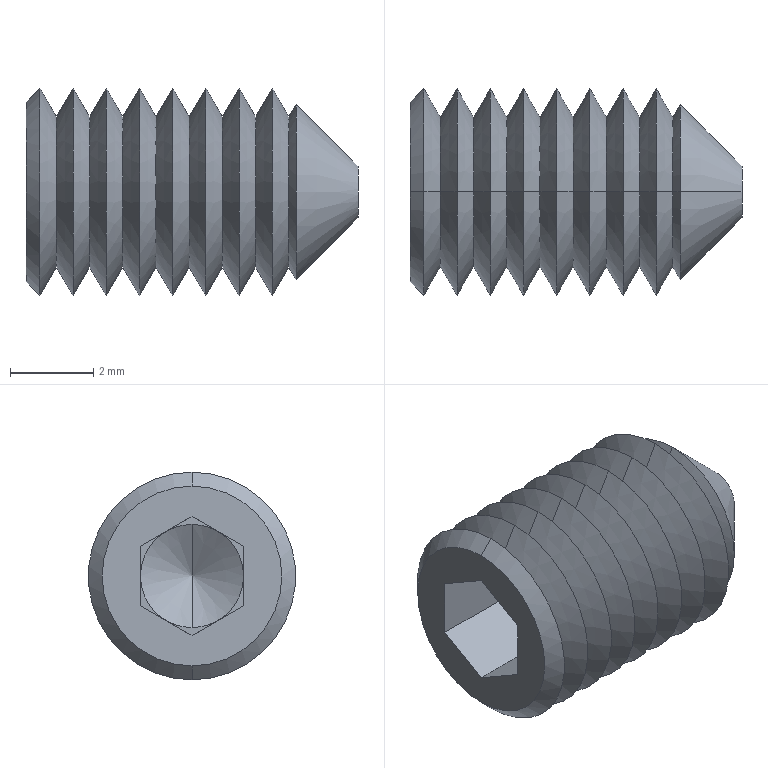Part | STEP file | GB/T 78 M5×8 | 1 solid | 52 faces | box 8 x 5 x 5 mm | volume 93.812 mm3 | cone 38 | plane 14
STEP:
#1=CARTESIAN_POINT('',(8.,0.,0.625));
#2=VERTEX_POINT('',#1);
#3=CARTESIAN_POINT('',(8.,0.,-0.625));
#4=VERTEX_POINT('',#3);
#5=CARTESIAN_POINT('',(8.,0.,0.));
#6=DIRECTION('',(-1.,0.,0.));
#7=DIRECTION('',(0.,0.,1.));
#8=AXIS2_PLACEMENT_3D('',#5,#6,#7);
#9=CIRCLE('',#8,0.625);
#10=EDGE_CURVE('',#2,#4,#9,.T.);
#11=ORIENTED_EDGE('',*,*,#10,.T.);
#12=CARTESIAN_POINT('',(6.51,0.,-2.115));
#13=VERTEX_POINT('',#12);
#14=CARTESIAN_POINT('',(8.,0.,-0.625));
#15=DIRECTION('',(-0.7071,0.,-0.7071));
#16=VECTOR('',#15,1000.);
#17=LINE('',#14,#16);
#18=EDGE_CURVE('',#4,#13,#17,.T.);
#19=ORIENTED_EDGE('',*,*,#18,.T.);
#20=CARTESIAN_POINT('',(6.51,0.,2.115));
#21=VERTEX_POINT('',#20);
#22=CARTESIAN_POINT('',(6.51,0.,0.));
#23=DIRECTION('',(-1.,0.,0.));
#24=DIRECTION('',(0.,0.,-1.));
#25=AXIS2_PLACEMENT_3D('',#22,#23,#24);
#26=CIRCLE('',#25,2.115);
#27=EDGE_CURVE('',#21,#13,#26,.T.);
#28=ORIENTED_EDGE('',*,*,#27,.F.);
#29=CARTESIAN_POINT('',(8.,0.,0.625));
#30=DIRECTION('',(-0.7071,0.,0.7071));
#31=VECTOR('',#30,1000.);
#32=LINE('',#29,#31);
#33=EDGE_CURVE('',#2,#21,#32,.T.);
#34=ORIENTED_EDGE('',*,*,#33,.F.);
#35=EDGE_LOOP('',(#11,#19,#28,#34));
#36=FACE_OUTER_BOUND('',#35,.T.);
#37=CARTESIAN_POINT('',(8.,0.,0.));
#38=DIRECTION('',(-1.,0.,0.));
#39=DIRECTION('',(0.,0.,1.));
#40=AXIS2_PLACEMENT_3D('',#37,#38,#39);
#41=CONICAL_SURFACE('',#40,0.625,0.7854);
#42=ADVANCED_FACE('',(#36),#41,.T.);
#43=CARTESIAN_POINT('',(6.331,0.,1.807));
#44=VERTEX_POINT('',#43);
#45=CARTESIAN_POINT('',(6.331,0.,-1.807));
#46=VERTEX_POINT('',#45);
#47=CARTESIAN_POINT('',(6.331,0.,0.));
#48=DIRECTION('',(-1.,0.,0.));
#49=DIRECTION('',(0.,0.,1.));
#50=AXIS2_PLACEMENT_3D('',#47,#48,#49);
#51=CIRCLE('',#50,1.807);
#52=EDGE_CURVE('',#44,#46,#51,.T.);
#53=ORIENTED_EDGE('',*,*,#52,.T.);
#54=CARTESIAN_POINT('',(5.935,0.,-2.5));
#55=VERTEX_POINT('',#54);
#56=CARTESIAN_POINT('',(5.935,0.,-2.5));
#57=DIRECTION('',(-0.4959,0.,-0.8684));
#58=VECTOR('',#57,1000.);
#59=LINE('',#56,#58);
#60=EDGE_CURVE('',#46,#55,#59,.T.);
#61=ORIENTED_EDGE('',*,*,#60,.T.);
#62=CARTESIAN_POINT('',(5.935,0.,2.5));
#63=VERTEX_POINT('',#62);
#64=CARTESIAN_POINT('',(5.935,0.,0.));
#65=DIRECTION('',(-1.,0.,0.));
#66=DIRECTION('',(0.,0.,1.));
#67=AXIS2_PLACEMENT_3D('',#64,#65,#66);
#68=CIRCLE('',#67,2.5);
#69=EDGE_CURVE('',#63,#55,#68,.T.);
#70=ORIENTED_EDGE('',*,*,#69,.F.);
#71=CARTESIAN_POINT('',(5.935,0.,2.5));
#72=DIRECTION('',(-0.4959,0.,0.8684));
#73=VECTOR('',#72,1000.);
#74=LINE('',#71,#73);
#75=EDGE_CURVE('',#44,#63,#74,.T.);
#76=ORIENTED_EDGE('',*,*,#75,.F.);
#77=EDGE_LOOP('',(#53,#61,#70,#76));
#78=FACE_OUTER_BOUND('',#77,.T.);
#79=CARTESIAN_POINT('',(5.935,0.,0.));
#80=DIRECTION('',(-1.,0.,0.));
#81=DIRECTION('',(0.,0.,1.));
#82=AXIS2_PLACEMENT_3D('',#79,#80,#81);
#83=CONICAL_SURFACE('',#82,2.5,1.052);
#84=ADVANCED_FACE('',(#78),#83,.T.);
#85=ORIENTED_EDGE('',*,*,#52,.F.);
#86=CARTESIAN_POINT('',(6.331,0.,1.807));
#87=DIRECTION('',(0.5041,0.,0.8637));
#88=VECTOR('',#87,1000.);
#89=LINE('',#86,#88);
#90=EDGE_CURVE('',#44,#21,#89,.T.);
#91=ORIENTED_EDGE('',*,*,#90,.T.);
#92=ORIENTED_EDGE('',*,*,#27,.T.);
#93=CARTESIAN_POINT('',(6.331,0.,-1.807));
#94=DIRECTION('',(0.5041,0.,-0.8637));
#95=VECTOR('',#94,1000.);
#96=LINE('',#93,#95);
#97=EDGE_CURVE('',#46,#13,#96,.T.);
#98=ORIENTED_EDGE('',*,*,#97,.F.);
#99=EDGE_LOOP('',(#85,#91,#92,#98));
#100=FACE_OUTER_BOUND('',#99,.T.);
#101=CARTESIAN_POINT('',(6.331,0.,0.));
#102=DIRECTION('',(1.,0.,0.));
#103=DIRECTION('',(0.,0.,-1.));
#104=AXIS2_PLACEMENT_3D('',#101,#102,#103);
#105=CONICAL_SURFACE('',#104,1.807,1.043);
#106=ADVANCED_FACE('',(#100),#105,.T.);
#107=CARTESIAN_POINT('',(5.531,0.,1.807));
#108=VERTEX_POINT('',#107);
#109=CARTESIAN_POINT('',(5.531,0.,-1.807));
#110=VERTEX_POINT('',#109);
#111=CARTESIAN_POINT('',(5.531,0.,0.));
#112=DIRECTION('',(-1.,0.,0.));
#113=DIRECTION('',(0.,0.,1.));
#114=AXIS2_PLACEMENT_3D('',#111,#112,#113);
#115=CIRCLE('',#114,1.807);
#116=EDGE_CURVE('',#108,#110,#115,.T.);
#117=ORIENTED_EDGE('',*,*,#116,.F.);
#118=CARTESIAN_POINT('',(5.531,0.,1.807));
#119=DIRECTION('',(0.5041,0.,0.8637));
#120=VECTOR('',#119,1000.);
#121=LINE('',#118,#120);
#122=EDGE_CURVE('',#108,#63,#121,.T.);
#123=ORIENTED_EDGE('',*,*,#122,.T.);
#124=ORIENTED_EDGE('',*,*,#69,.T.);
#125=CARTESIAN_POINT('',(5.531,0.,-1.807));
#126=DIRECTION('',(0.5041,0.,-0.8637));
#127=VECTOR('',#126,1000.);
#128=LINE('',#125,#127);
#129=EDGE_CURVE('',#110,#55,#128,.T.);
#130=ORIENTED_EDGE('',*,*,#129,.F.);
#131=EDGE_LOOP('',(#117,#123,#124,#130));
#132=FACE_OUTER_BOUND('',#131,.T.);
#133=CARTESIAN_POINT('',(5.531,0.,0.));
#134=DIRECTION('',(1.,0.,0.));
#135=DIRECTION('',(0.,0.,-1.));
#136=AXIS2_PLACEMENT_3D('',#133,#134,#135);
#137=CONICAL_SURFACE('',#136,1.807,1.043);
#138=ADVANCED_FACE('',(#132),#137,.T.);
#139=ORIENTED_EDGE('',*,*,#116,.T.);
#140=CARTESIAN_POINT('',(5.135,0.,-2.5));
#141=VERTEX_POINT('',#140);
#142=CARTESIAN_POINT('',(5.135,0.,-2.5));
#143=DIRECTION('',(-0.4959,0.,-0.8684));
#144=VECTOR('',#143,1000.);
#145=LINE('',#142,#144);
#146=EDGE_CURVE('',#110,#141,#145,.T.);
#147=ORIENTED_EDGE('',*,*,#146,.T.);
#148=CARTESIAN_POINT('',(5.135,0.,2.5));
#149=VERTEX_POINT('',#148);
#150=CARTESIAN_POINT('',(5.135,0.,0.));
#151=DIRECTION('',(-1.,0.,0.));
#152=DIRECTION('',(0.,0.,1.));
#153=AXIS2_PLACEMENT_3D('',#150,#151,#152);
#154=CIRCLE('',#153,2.5);
#155=EDGE_CURVE('',#149,#141,#154,.T.);
#156=ORIENTED_EDGE('',*,*,#155,.F.);
#157=CARTESIAN_POINT('',(5.135,0.,2.5));
#158=DIRECTION('',(-0.4959,0.,0.8684));
#159=VECTOR('',#158,1000.);
#160=LINE('',#157,#159);
#161=EDGE_CURVE('',#108,#149,#160,.T.);
#162=ORIENTED_EDGE('',*,*,#161,.F.);
#163=EDGE_LOOP('',(#139,#147,#156,#162));
#164=FACE_OUTER_BOUND('',#163,.T.);
#165=CARTESIAN_POINT('',(5.135,0.,0.));
#166=DIRECTION('',(-1.,0.,0.));
#167=DIRECTION('',(0.,0.,1.));
#168=AXIS2_PLACEMENT_3D('',#165,#166,#167);
#169=CONICAL_SURFACE('',#168,2.5,1.052);
#170=ADVANCED_FACE('',(#164),#169,.T.);
#171=CARTESIAN_POINT('',(4.731,0.,1.807));
#172=VERTEX_POINT('',#171);
#173=CARTESIAN_POINT('',(4.731,0.,-1.807));
#174=VERTEX_POINT('',#173);
#175=CARTESIAN_POINT('',(4.731,0.,0.));
#176=DIRECTION('',(-1.,0.,0.));
#177=DIRECTION('',(0.,0.,1.));
#178=AXIS2_PLACEMENT_3D('',#175,#176,#177);
#179=CIRCLE('',#178,1.807);
#180=EDGE_CURVE('',#172,#174,#179,.T.);
#181=ORIENTED_EDGE('',*,*,#180,.F.);
#182=CARTESIAN_POINT('',(4.731,0.,1.807));
#183=DIRECTION('',(0.5041,0.,0.8637));
#184=VECTOR('',#183,1000.);
#185=LINE('',#182,#184);
#186=EDGE_CURVE('',#172,#149,#185,.T.);
#187=ORIENTED_EDGE('',*,*,#186,.T.);
#188=ORIENTED_EDGE('',*,*,#155,.T.);
#189=CARTESIAN_POINT('',(4.731,0.,-1.807));
#190=DIRECTION('',(0.5041,0.,-0.8637));
#191=VECTOR('',#190,1000.);
#192=LINE('',#189,#191);
#193=EDGE_CURVE('',#174,#141,#192,.T.);
#194=ORIENTED_EDGE('',*,*,#193,.F.);
#195=EDGE_LOOP('',(#181,#187,#188,#194));
#196=FACE_OUTER_BOUND('',#195,.T.);
#197=CARTESIAN_POINT('',(4.731,0.,0.));
#198=DIRECTION('',(1.,0.,0.));
#199=DIRECTION('',(0.,0.,-1.));
#200=AXIS2_PLACEMENT_3D('',#197,#198,#199);
#201=CONICAL_SURFACE('',#200,1.807,1.043);
#202=ADVANCED_FACE('',(#196),#201,.T.);
#203=ORIENTED_EDGE('',*,*,#180,.T.);
#204=CARTESIAN_POINT('',(4.335,0.,-2.5));
#205=VERTEX_POINT('',#204);
#206=CARTESIAN_POINT('',(4.335,0.,-2.5));
#207=DIRECTION('',(-0.4959,0.,-0.8684));
#208=VECTOR('',#207,1000.);
#209=LINE('',#206,#208);
#210=EDGE_CURVE('',#174,#205,#209,.T.);
#211=ORIENTED_EDGE('',*,*,#210,.T.);
#212=CARTESIAN_POINT('',(4.335,0.,2.5));
#213=VERTEX_POINT('',#212);
#214=CARTESIAN_POINT('',(4.335,0.,0.));
#215=DIRECTION('',(-1.,0.,0.));
#216=DIRECTION('',(0.,0.,1.));
#217=AXIS2_PLACEMENT_3D('',#214,#215,#216);
#218=CIRCLE('',#217,2.5);
#219=EDGE_CURVE('',#213,#205,#218,.T.);
#220=ORIENTED_EDGE('',*,*,#219,.F.);
#221=CARTESIAN_POINT('',(4.335,0.,2.5));
#222=DIRECTION('',(-0.4959,0.,0.8684));
#223=VECTOR('',#222,1000.);
#224=LINE('',#221,#223);
#225=EDGE_CURVE('',#172,#213,#224,.T.);
#226=ORIENTED_EDGE('',*,*,#225,.F.);
#227=EDGE_LOOP('',(#203,#211,#220,#226));
#228=FACE_OUTER_BOUND('',#227,.T.);
#229=CARTESIAN_POINT('',(4.335,0.,0.));
#230=DIRECTION('',(-1.,0.,0.));
#231=DIRECTION('',(0.,0.,1.));
#232=AXIS2_PLACEMENT_3D('',#229,#230,#231);
#233=CONICAL_SURFACE('',#232,2.5,1.052);
#234=ADVANCED_FACE('',(#228),#233,.T.);
#235=CARTESIAN_POINT('',(3.931,0.,1.807));
#236=VERTEX_POINT('',#235);
#237=CARTESIAN_POINT('',(3.931,0.,-1.807));
#238=VERTEX_POINT('',#237);
#239=CARTESIAN_POINT('',(3.931,0.,0.));
#240=DIRECTION('',(-1.,0.,0.));
#241=DIRECTION('',(0.,0.,1.));
#242=AXIS2_PLACEMENT_3D('',#239,#240,#241);
#243=CIRCLE('',#242,1.807);
#244=EDGE_CURVE('',#236,#238,#243,.T.);
#245=ORIENTED_EDGE('',*,*,#244,.F.);
#246=CARTESIAN_POINT('',(3.931,0.,1.807));
#247=DIRECTION('',(0.5041,0.,0.8637));
#248=VECTOR('',#247,1000.);
#249=LINE('',#246,#248);
#250=EDGE_CURVE('',#236,#213,#249,.T.);
#251=ORIENTED_EDGE('',*,*,#250,.T.);
#252=ORIENTED_EDGE('',*,*,#219,.T.);
#253=CARTESIAN_POINT('',(3.931,0.,-1.807));
#254=DIRECTION('',(0.5041,0.,-0.8637));
#255=VECTOR('',#254,1000.);
#256=LINE('',#253,#255);
#257=EDGE_CURVE('',#238,#205,#256,.T.);
#258=ORIENTED_EDGE('',*,*,#257,.F.);
#259=EDGE_LOOP('',(#245,#251,#252,#258));
#260=FACE_OUTER_BOUND('',#259,.T.);
#261=CARTESIAN_POINT('',(3.931,0.,0.));
#262=DIRECTION('',(1.,0.,0.));
#263=DIRECTION('',(0.,0.,-1.));
#264=AXIS2_PLACEMENT_3D('',#261,#262,#263);
#265=CONICAL_SURFACE('',#264,1.807,1.043);
#266=ADVANCED_FACE('',(#260),#265,.T.);
#267=ORIENTED_EDGE('',*,*,#244,.T.);
#268=CARTESIAN_POINT('',(3.535,0.,-2.5));
#269=VERTEX_POINT('',#268);
#270=CARTESIAN_POINT('',(3.535,0.,-2.5));
#271=DIRECTION('',(-0.4959,0.,-0.8684));
#272=VECTOR('',#271,1000.);
#273=LINE('',#270,#272);
#274=EDGE_CURVE('',#238,#269,#273,.T.);
#275=ORIENTED_EDGE('',*,*,#274,.T.);
#276=CARTESIAN_POINT('',(3.535,0.,2.5));
#277=VERTEX_POINT('',#276);
#278=CARTESIAN_POINT('',(3.535,0.,0.));
#279=DIRECTION('',(-1.,0.,0.));
#280=DIRECTION('',(0.,0.,1.));
#281=AXIS2_PLACEMENT_3D('',#278,#279,#280);
#282=CIRCLE('',#281,2.5);
#283=EDGE_CURVE('',#277,#269,#282,.T.);
#284=ORIENTED_EDGE('',*,*,#283,.F.);
#285=CARTESIAN_POINT('',(3.535,0.,2.5));
#286=DIRECTION('',(-0.4959,0.,0.8684));
#287=VECTOR('',#286,1000.);
#288=LINE('',#285,#287);
#289=EDGE_CURVE('',#236,#277,#288,.T.);
#290=ORIENTED_EDGE('',*,*,#289,.F.);
#291=EDGE_LOOP('',(#267,#275,#284,#290));
#292=FACE_OUTER_BOUND('',#291,.T.);
#293=CARTESIAN_POINT('',(3.535,0.,0.));
#294=DIRECTION('',(-1.,0.,0.));
#295=DIRECTION('',(0.,0.,1.));
#296=AXIS2_PLACEMENT_3D('',#293,#294,#295);
#297=CONICAL_SURFACE('',#296,2.5,1.052);
#298=ADVANCED_FACE('',(#292),#297,.T.);
#299=CARTESIAN_POINT('',(3.131,0.,1.807));
#300=VERTEX_POINT('',#299);
#301=CARTESIAN_POINT('',(3.131,0.,-1.807));
#302=VERTEX_POINT('',#301);
#303=CARTESIAN_POINT('',(3.131,0.,0.));
#304=DIRECTION('',(-1.,0.,0.));
#305=DIRECTION('',(0.,0.,1.));
#306=AXIS2_PLACEMENT_3D('',#303,#304,#305);
#307=CIRCLE('',#306,1.807);
#308=EDGE_CURVE('',#300,#302,#307,.T.);
#309=ORIENTED_EDGE('',*,*,#308,.F.);
#310=CARTESIAN_POINT('',(3.131,0.,1.807));
#311=DIRECTION('',(0.5041,0.,0.8637));
#312=VECTOR('',#311,1000.);
#313=LINE('',#310,#312);
#314=EDGE_CURVE('',#300,#277,#313,.T.);
#315=ORIENTED_EDGE('',*,*,#314,.T.);
#316=ORIENTED_EDGE('',*,*,#283,.T.);
#317=CARTESIAN_POINT('',(3.131,0.,-1.807));
#318=DIRECTION('',(0.5041,0.,-0.8637));
#319=VECTOR('',#318,1000.);
#320=LINE('',#317,#319);
#321=EDGE_CURVE('',#302,#269,#320,.T.);
#322=ORIENTED_EDGE('',*,*,#321,.F.);
#323=EDGE_LOOP('',(#309,#315,#316,#322));
#324=FACE_OUTER_BOUND('',#323,.T.);
#325=CARTESIAN_POINT('',(3.131,0.,0.));
#326=DIRECTION('',(1.,0.,0.));
#327=DIRECTION('',(0.,0.,-1.));
#328=AXIS2_PLACEMENT_3D('',#325,#326,#327);
#329=CONICAL_SURFACE('',#328,1.807,1.043);
#330=ADVANCED_FACE('',(#324),#329,.T.);
#331=ORIENTED_EDGE('',*,*,#308,.T.);
#332=CARTESIAN_POINT('',(2.735,0.,-2.5));
#333=VERTEX_POINT('',#332);
#334=CARTESIAN_POINT('',(2.735,0.,-2.5));
#335=DIRECTION('',(-0.4959,0.,-0.8684));
#336=VECTOR('',#335,1000.);
#337=LINE('',#334,#336);
#338=EDGE_CURVE('',#302,#333,#337,.T.);
#339=ORIENTED_EDGE('',*,*,#338,.T.);
#340=CARTESIAN_POINT('',(2.735,0.,2.5));
#341=VERTEX_POINT('',#340);
#342=CARTESIAN_POINT('',(2.735,0.,0.));
#343=DIRECTION('',(-1.,0.,0.));
#344=DIRECTION('',(0.,0.,1.));
#345=AXIS2_PLACEMENT_3D('',#342,#343,#344);
#346=CIRCLE('',#345,2.5);
#347=EDGE_CURVE('',#341,#333,#346,.T.);
#348=ORIENTED_EDGE('',*,*,#347,.F.);
#349=CARTESIAN_POINT('',(2.735,0.,2.5));
#350=DIRECTION('',(-0.4959,0.,0.8684));
#351=VECTOR('',#350,1000.);
#352=LINE('',#349,#351);
#353=EDGE_CURVE('',#300,#341,#352,.T.);
#354=ORIENTED_EDGE('',*,*,#353,.F.);
#355=EDGE_LOOP('',(#331,#339,#348,#354));
#356=FACE_OUTER_BOUND('',#355,.T.);
#357=CARTESIAN_POINT('',(2.735,0.,0.));
#358=DIRECTION('',(-1.,0.,0.));
#359=DIRECTION('',(0.,0.,1.));
#360=AXIS2_PLACEMENT_3D('',#357,#358,#359);
#361=CONICAL_SURFACE('',#360,2.5,1.052);
#362=ADVANCED_FACE('',(#356),#361,.T.);
#363=CARTESIAN_POINT('',(2.331,0.,1.807));
#364=VERTEX_POINT('',#363);
#365=CARTESIAN_POINT('',(2.331,0.,-1.807));
#366=VERTEX_POINT('',#365);
#367=CARTESIAN_POINT('',(2.331,0.,0.));
#368=DIRECTION('',(-1.,0.,0.));
#369=DIRECTION('',(0.,0.,1.));
#370=AXIS2_PLACEMENT_3D('',#367,#368,#369);
#371=CIRCLE('',#370,1.807);
#372=EDGE_CURVE('',#364,#366,#371,.T.);
#373=ORIENTED_EDGE('',*,*,#372,.F.);
#374=CARTESIAN_POINT('',(2.331,0.,1.807));
#375=DIRECTION('',(0.5041,0.,0.8637));
#376=VECTOR('',#375,1000.);
#377=LINE('',#374,#376);
#378=EDGE_CURVE('',#364,#341,#377,.T.);
#379=ORIENTED_EDGE('',*,*,#378,.T.);
#380=ORIENTED_EDGE('',*,*,#347,.T.);
#381=CARTESIAN_POINT('',(2.331,0.,-1.807));
#382=DIRECTION('',(0.5041,0.,-0.8637));
#383=VECTOR('',#382,1000.);
#384=LINE('',#381,#383);
#385=EDGE_CURVE('',#366,#333,#384,.T.);
#386=ORIENTED_EDGE('',*,*,#385,.F.);
#387=EDGE_LOOP('',(#373,#379,#380,#386));
#388=FACE_OUTER_BOUND('',#387,.T.);
#389=CARTESIAN_POINT('',(2.331,0.,0.));
#390=DIRECTION('',(1.,0.,0.));
#391=DIRECTION('',(0.,0.,-1.));
#392=AXIS2_PLACEMENT_3D('',#389,#390,#391);
#393=CONICAL_SURFACE('',#392,1.807,1.043);
#394=ADVANCED_FACE('',(#388),#393,.T.);
#395=ORIENTED_EDGE('',*,*,#372,.T.);
#396=CARTESIAN_POINT('',(1.935,0.,-2.5));
#397=VERTEX_POINT('',#396);
#398=CARTESIAN_POINT('',(1.935,0.,-2.5));
#399=DIRECTION('',(-0.4959,0.,-0.8684));
#400=VECTOR('',#399,1000.);
#401=LINE('',#398,#400);
#402=EDGE_CURVE('',#366,#397,#401,.T.);
#403=ORIENTED_EDGE('',*,*,#402,.T.);
#404=CARTESIAN_POINT('',(1.935,0.,2.5));
#405=VERTEX_POINT('',#404);
#406=CARTESIAN_POINT('',(1.935,0.,0.));
#407=DIRECTION('',(-1.,0.,0.));
#408=DIRECTION('',(0.,0.,1.));
#409=AXIS2_PLACEMENT_3D('',#406,#407,#408);
#410=CIRCLE('',#409,2.5);
#411=EDGE_CURVE('',#405,#397,#410,.T.);
#412=ORIENTED_EDGE('',*,*,#411,.F.);
#413=CARTESIAN_POINT('',(1.935,0.,2.5));
#414=DIRECTION('',(-0.4959,0.,0.8684));
#415=VECTOR('',#414,1000.);
#416=LINE('',#413,#415);
#417=EDGE_CURVE('',#364,#405,#416,.T.);
#418=ORIENTED_EDGE('',*,*,#417,.F.);
#419=EDGE_LOOP('',(#395,#403,#412,#418));
#420=FACE_OUTER_BOUND('',#419,.T.);
#421=CARTESIAN_POINT('',(1.935,0.,0.));
#422=DIRECTION('',(-1.,0.,0.));
#423=DIRECTION('',(0.,0.,1.));
#424=AXIS2_PLACEMENT_3D('',#421,#422,#423);
#425=CONICAL_SURFACE('',#424,2.5,1.052);
#426=ADVANCED_FACE('',(#420),#425,.T.);
#427=CARTESIAN_POINT('',(1.531,0.,1.807));
#428=VERTEX_POINT('',#427);
#429=CARTESIAN_POINT('',(1.531,0.,-1.807));
#430=VERTEX_POINT('',#429);
#431=CARTESIAN_POINT('',(1.531,0.,0.));
#432=DIRECTION('',(-1.,0.,0.));
#433=DIRECTION('',(0.,0.,1.));
#434=AXIS2_PLACEMENT_3D('',#431,#432,#433);
#435=CIRCLE('',#434,1.807);
#436=EDGE_CURVE('',#428,#430,#435,.T.);
#437=ORIENTED_EDGE('',*,*,#436,.F.);
#438=CARTESIAN_POINT('',(1.531,0.,1.807));
#439=DIRECTION('',(0.5041,0.,0.8637));
#440=VECTOR('',#439,1000.);
#441=LINE('',#438,#440);
#442=EDGE_CURVE('',#428,#405,#441,.T.);
#443=ORIENTED_EDGE('',*,*,#442,.T.);
#444=ORIENTED_EDGE('',*,*,#411,.T.);
#445=CARTESIAN_POINT('',(1.531,0.,-1.807));
#446=DIRECTION('',(0.5041,0.,-0.8637));
#447=VECTOR('',#446,1000.);
#448=LINE('',#445,#447);
#449=EDGE_CURVE('',#430,#397,#448,.T.);
#450=ORIENTED_EDGE('',*,*,#449,.F.);
#451=EDGE_LOOP('',(#437,#443,#444,#450));
#452=FACE_OUTER_BOUND('',#451,.T.);
#453=CARTESIAN_POINT('',(1.531,0.,0.));
#454=DIRECTION('',(1.,0.,0.));
#455=DIRECTION('',(0.,0.,-1.));
#456=AXIS2_PLACEMENT_3D('',#453,#454,#455);
#457=CONICAL_SURFACE('',#456,1.807,1.043);
#458=ADVANCED_FACE('',(#452),#457,.T.);
#459=ORIENTED_EDGE('',*,*,#436,.T.);
#460=CARTESIAN_POINT('',(1.135,0.,-2.5));
#461=VERTEX_POINT('',#460);
#462=CARTESIAN_POINT('',(1.135,0.,-2.5));
#463=DIRECTION('',(-0.4959,0.,-0.8684));
#464=VECTOR('',#463,1000.);
#465=LINE('',#462,#464);
#466=EDGE_CURVE('',#430,#461,#465,.T.);
#467=ORIENTED_EDGE('',*,*,#466,.T.);
#468=CARTESIAN_POINT('',(1.135,0.,2.5));
#469=VERTEX_POINT('',#468);
#470=CARTESIAN_POINT('',(1.135,0.,0.));
#471=DIRECTION('',(-1.,0.,0.));
#472=DIRECTION('',(0.,0.,1.));
#473=AXIS2_PLACEMENT_3D('',#470,#471,#472);
#474=CIRCLE('',#473,2.5);
#475=EDGE_CURVE('',#469,#461,#474,.T.);
#476=ORIENTED_EDGE('',*,*,#475,.F.);
#477=CARTESIAN_POINT('',(1.135,0.,2.5));
#478=DIRECTION('',(-0.4959,0.,0.8684));
#479=VECTOR('',#478,1000.);
#480=LINE('',#477,#479);
#481=EDGE_CURVE('',#428,#469,#480,.T.);
#482=ORIENTED_EDGE('',*,*,#481,.F.);
#483=EDGE_LOOP('',(#459,#467,#476,#482));
#484=FACE_OUTER_BOUND('',#483,.T.);
#485=CARTESIAN_POINT('',(1.135,0.,0.));
#486=DIRECTION('',(-1.,0.,0.));
#487=DIRECTION('',(0.,0.,1.));
#488=AXIS2_PLACEMENT_3D('',#485,#486,#487);
#489=CONICAL_SURFACE('',#488,2.5,1.052);
#490=ADVANCED_FACE('',(#484),#489,.T.);
#491=CARTESIAN_POINT('',(0.7307,0.,1.807));
#492=VERTEX_POINT('',#491);
#493=CARTESIAN_POINT('',(0.7307,0.,-1.807));
#494=VERTEX_POINT('',#493);
#495=CARTESIAN_POINT('',(0.7307,0.,0.));
#496=DIRECTION('',(-1.,0.,0.));
#497=DIRECTION('',(0.,0.,1.));
#498=AXIS2_PLACEMENT_3D('',#495,#496,#497);
#499=CIRCLE('',#498,1.807);
#500=EDGE_CURVE('',#492,#494,#499,.T.);
#501=ORIENTED_EDGE('',*,*,#500,.F.);
#502=CARTESIAN_POINT('',(0.7307,0.,1.807));
#503=DIRECTION('',(0.5041,0.,0.8637));
#504=VECTOR('',#503,1000.);
#505=LINE('',#502,#504);
#506=EDGE_CURVE('',#492,#469,#505,.T.);
#507=ORIENTED_EDGE('',*,*,#506,.T.);
#508=ORIENTED_EDGE('',*,*,#475,.T.);
#509=CARTESIAN_POINT('',(0.7307,0.,-1.807));
#510=DIRECTION('',(0.5041,0.,-0.8637));
#511=VECTOR('',#510,1000.);
#512=LINE('',#509,#511);
#513=EDGE_CURVE('',#494,#461,#512,.T.);
#514=ORIENTED_EDGE('',*,*,#513,.F.);
#515=EDGE_LOOP('',(#501,#507,#508,#514));
#516=FACE_OUTER_BOUND('',#515,.T.);
#517=CARTESIAN_POINT('',(0.7307,0.,0.));
#518=DIRECTION('',(1.,0.,0.));
#519=DIRECTION('',(0.,0.,-1.));
#520=AXIS2_PLACEMENT_3D('',#517,#518,#519);
#521=CONICAL_SURFACE('',#520,1.807,1.043);
#522=ADVANCED_FACE('',(#516),#521,.T.);
#523=ORIENTED_EDGE('',*,*,#500,.T.);
#524=CARTESIAN_POINT('',(0.335,0.,-2.5));
#525=VERTEX_POINT('',#524);
#526=CARTESIAN_POINT('',(0.335,0.,-2.5));
#527=DIRECTION('',(-0.4959,0.,-0.8684));
#528=VECTOR('',#527,1000.);
#529=LINE('',#526,#528);
#530=EDGE_CURVE('',#494,#525,#529,.T.);
#531=ORIENTED_EDGE('',*,*,#530,.T.);
#532=CARTESIAN_POINT('',(0.335,0.,2.5));
#533=VERTEX_POINT('',#532);
#534=CARTESIAN_POINT('',(0.335,0.,0.));
#535=DIRECTION('',(-1.,0.,0.));
#536=DIRECTION('',(0.,0.,1.));
#537=AXIS2_PLACEMENT_3D('',#534,#535,#536);
#538=CIRCLE('',#537,2.5);
#539=EDGE_CURVE('',#533,#525,#538,.T.);
#540=ORIENTED_EDGE('',*,*,#539,.F.);
#541=CARTESIAN_POINT('',(0.335,0.,2.5));
#542=DIRECTION('',(-0.4959,0.,0.8684));
#543=VECTOR('',#542,1000.);
#544=LINE('',#541,#543);
#545=EDGE_CURVE('',#492,#533,#544,.T.);
#546=ORIENTED_EDGE('',*,*,#545,.F.);
#547=EDGE_LOOP('',(#523,#531,#540,#546));
#548=FACE_OUTER_BOUND('',#547,.T.);
#549=CARTESIAN_POINT('',(0.335,0.,0.));
#550=DIRECTION('',(-1.,0.,0.));
#551=DIRECTION('',(0.,0.,1.));
#552=AXIS2_PLACEMENT_3D('',#549,#550,#551);
#553=CONICAL_SURFACE('',#552,2.5,1.052);
#554=ADVANCED_FACE('',(#548),#553,.T.);
#555=CARTESIAN_POINT('',(2.718,0.,0.));
#556=VERTEX_POINT('',#555);
#557=CARTESIAN_POINT('',(2.,0.,1.243));
#558=VERTEX_POINT('',#557);
#559=CARTESIAN_POINT('',(2.718,0.,0.));
#560=DIRECTION('',(-0.5,0.,0.866));
#561=VECTOR('',#560,1000.);
#562=LINE('',#559,#561);
#563=EDGE_CURVE('',#556,#558,#562,.T.);
#564=ORIENTED_EDGE('',*,*,#563,.F.);
#565=CARTESIAN_POINT('',(2.,0.,-1.243));
#566=VERTEX_POINT('',#565);
#567=CARTESIAN_POINT('',(2.718,0.,0.));
#568=DIRECTION('',(-0.5,0.,-0.866));
#569=VECTOR('',#568,1000.);
#570=LINE('',#567,#569);
#571=EDGE_CURVE('',#556,#566,#570,.T.);
#572=ORIENTED_EDGE('',*,*,#571,.T.);
#573=CARTESIAN_POINT('',(2.,-0.6214,-1.076));
#574=VERTEX_POINT('',#573);
#575=CARTESIAN_POINT('',(2.,0.,0.));
#576=DIRECTION('',(-1.,0.,0.));
#577=DIRECTION('',(0.,0.,1.));
#578=AXIS2_PLACEMENT_3D('',#575,#576,#577);
#579=CIRCLE('',#578,1.243);
#580=EDGE_CURVE('',#566,#574,#579,.T.);
#581=ORIENTED_EDGE('',*,*,#580,.T.);
#582=CARTESIAN_POINT('',(2.,-1.243,0.));
#583=VERTEX_POINT('',#582);
#584=CARTESIAN_POINT('',(2.,0.,0.));
#585=DIRECTION('',(-1.,0.,0.));
#586=DIRECTION('',(0.,0.,1.));
#587=AXIS2_PLACEMENT_3D('',#584,#585,#586);
#588=CIRCLE('',#587,1.243);
#589=EDGE_CURVE('',#574,#583,#588,.T.);
#590=ORIENTED_EDGE('',*,*,#589,.T.);
#591=CARTESIAN_POINT('',(2.,-0.6214,1.076));
#592=VERTEX_POINT('',#591);
#593=CARTESIAN_POINT('',(2.,0.,0.));
#594=DIRECTION('',(-1.,0.,0.));
#595=DIRECTION('',(0.,0.,1.));
#596=AXIS2_PLACEMENT_3D('',#593,#594,#595);
#597=CIRCLE('',#596,1.243);
#598=EDGE_CURVE('',#583,#592,#597,.T.);
#599=ORIENTED_EDGE('',*,*,#598,.T.);
#600=CARTESIAN_POINT('',(2.,0.,0.));
#601=DIRECTION('',(-1.,0.,0.));
#602=DIRECTION('',(0.,0.,1.));
#603=AXIS2_PLACEMENT_3D('',#600,#601,#602);
#604=CIRCLE('',#603,1.243);
#605=EDGE_CURVE('',#592,#558,#604,.T.);
#606=ORIENTED_EDGE('',*,*,#605,.T.);
#607=EDGE_LOOP('',(#564,#572,#581,#590,#599,#606));
#608=FACE_OUTER_BOUND('',#607,.T.);
#609=CARTESIAN_POINT('',(-997.282,0.,0.));
#610=DIRECTION('',(-1.,0.,0.));
#611=DIRECTION('',(0.,0.,1.));
#612=AXIS2_PLACEMENT_3D('',#609,#610,#611);
#613=CONICAL_SURFACE('',#612,1732.051,1.047);
#614=ADVANCED_FACE('',(#608),#613,.F.);
#615=CARTESIAN_POINT('',(0.,0.,2.165));
#616=VERTEX_POINT('',#615);
#617=CARTESIAN_POINT('',(0.,0.,-2.165));
#618=VERTEX_POINT('',#617);
#619=CARTESIAN_POINT('',(0.,0.,0.));
#620=DIRECTION('',(-1.,0.,0.));
#621=DIRECTION('',(0.,0.,1.));
#622=AXIS2_PLACEMENT_3D('',#619,#620,#621);
#623=CIRCLE('',#622,2.165);
#624=EDGE_CURVE('',#616,#618,#623,.T.);
#625=ORIENTED_EDGE('',*,*,#624,.F.);
#626=CARTESIAN_POINT('',(0.335,0.,2.5));
#627=DIRECTION('',(0.7071,0.,0.7071));
#628=VECTOR('',#627,1000.);
#629=LINE('',#626,#628);
#630=EDGE_CURVE('',#616,#533,#629,.T.);
#631=ORIENTED_EDGE('',*,*,#630,.T.);
#632=ORIENTED_EDGE('',*,*,#539,.T.);
#633=CARTESIAN_POINT('',(0.335,0.,-2.5));
#634=DIRECTION('',(0.7071,0.,-0.7071));
#635=VECTOR('',#634,1000.);
#636=LINE('',#633,#635);
#637=EDGE_CURVE('',#618,#525,#636,.T.);
#638=ORIENTED_EDGE('',*,*,#637,.F.);
#639=EDGE_LOOP('',(#625,#631,#632,#638));
#640=FACE_OUTER_BOUND('',#639,.T.);
#641=CARTESIAN_POINT('',(0.335,0.,0.));
#642=DIRECTION('',(1.,0.,0.));
#643=DIRECTION('',(0.,0.,-1.));
#644=AXIS2_PLACEMENT_3D('',#641,#642,#643);
#645=CONICAL_SURFACE('',#644,2.5,0.7854);
#646=ADVANCED_FACE('',(#640),#645,.T.);
#647=CARTESIAN_POINT('',(2.,0.6214,1.076));
#648=VERTEX_POINT('',#647);
#649=CARTESIAN_POINT('',(2.,1.243,0.));
#650=VERTEX_POINT('',#649);
#651=CARTESIAN_POINT('',(2.,0.,0.));
#652=DIRECTION('',(-1.,0.,0.));
#653=DIRECTION('',(0.,0.,1.));
#654=AXIS2_PLACEMENT_3D('',#651,#652,#653);
#655=CIRCLE('',#654,1.243);
#656=EDGE_CURVE('',#648,#650,#655,.T.);
#657=ORIENTED_EDGE('',*,*,#656,.F.);
#658=CARTESIAN_POINT('',(2.,1.243,0.7175));
#659=VERTEX_POINT('',#658);
#660=CARTESIAN_POINT('',(2.,0.,1.435));
#661=DIRECTION('',(0.,0.866,-0.5));
#662=VECTOR('',#661,1000.);
#663=LINE('',#660,#662);
#664=EDGE_CURVE('',#648,#659,#663,.T.);
#665=ORIENTED_EDGE('',*,*,#664,.T.);
#666=CARTESIAN_POINT('',(2.,1.243,0.7175));
#667=DIRECTION('',(0.,0.,-1.));
#668=VECTOR('',#667,1000.);
#669=LINE('',#666,#668);
#670=EDGE_CURVE('',#659,#650,#669,.T.);
#671=ORIENTED_EDGE('',*,*,#670,.T.);
#672=EDGE_LOOP('',(#657,#665,#671));
#673=FACE_OUTER_BOUND('',#672,.T.);
#674=CARTESIAN_POINT('',(2.,-1.243,0.7175));
#675=DIRECTION('',(1.,0.,0.));
#676=DIRECTION('',(0.,0.,-1.));
#677=AXIS2_PLACEMENT_3D('',#674,#675,#676);
#678=PLANE('',#677);
#679=ADVANCED_FACE('',(#673),#678,.F.);
#680=CARTESIAN_POINT('',(2.,0.6214,-1.076));
#681=VERTEX_POINT('',#680);
#682=CARTESIAN_POINT('',(2.,0.,0.));
#683=DIRECTION('',(-1.,0.,0.));
#684=DIRECTION('',(0.,0.,1.));
#685=AXIS2_PLACEMENT_3D('',#682,#683,#684);
#686=CIRCLE('',#685,1.243);
#687=EDGE_CURVE('',#650,#681,#686,.T.);
#688=ORIENTED_EDGE('',*,*,#687,.F.);
#689=CARTESIAN_POINT('',(2.,1.243,-0.7175));
#690=VERTEX_POINT('',#689);
#691=CARTESIAN_POINT('',(2.,1.243,0.7175));
#692=DIRECTION('',(0.,0.,-1.));
#693=VECTOR('',#692,1000.);
#694=LINE('',#691,#693);
#695=EDGE_CURVE('',#650,#690,#694,.T.);
#696=ORIENTED_EDGE('',*,*,#695,.T.);
#697=CARTESIAN_POINT('',(2.,1.243,-0.7175));
#698=DIRECTION('',(0.,-0.866,-0.5));
#699=VECTOR('',#698,1000.);
#700=LINE('',#697,#699);
#701=EDGE_CURVE('',#690,#681,#700,.T.);
#702=ORIENTED_EDGE('',*,*,#701,.T.);
#703=EDGE_LOOP('',(#688,#696,#702));
#704=FACE_OUTER_BOUND('',#703,.T.);
#705=CARTESIAN_POINT('',(2.,-1.243,0.7175));
#706=DIRECTION('',(1.,0.,0.));
#707=DIRECTION('',(0.,0.,-1.));
#708=AXIS2_PLACEMENT_3D('',#705,#706,#707);
#709=PLANE('',#708);
#710=ADVANCED_FACE('',(#704),#709,.F.);
#711=CARTESIAN_POINT('',(2.,0.,0.));
#712=DIRECTION('',(-1.,0.,0.));
#713=DIRECTION('',(0.,0.,1.));
#714=AXIS2_PLACEMENT_3D('',#711,#712,#713);
#715=CIRCLE('',#714,1.243);
#716=EDGE_CURVE('',#681,#566,#715,.T.);
#717=ORIENTED_EDGE('',*,*,#716,.F.);
#718=CARTESIAN_POINT('',(2.,0.,-1.435));
#719=VERTEX_POINT('',#718);
#720=CARTESIAN_POINT('',(2.,1.243,-0.7175));
#721=DIRECTION('',(0.,-0.866,-0.5));
#722=VECTOR('',#721,1000.);
#723=LINE('',#720,#722);
#724=EDGE_CURVE('',#681,#719,#723,.T.);
#725=ORIENTED_EDGE('',*,*,#724,.T.);
#726=CARTESIAN_POINT('',(2.,0.,-1.435));
#727=DIRECTION('',(0.,-0.866,0.5));
#728=VECTOR('',#727,1000.);
#729=LINE('',#726,#728);
#730=EDGE_CURVE('',#719,#574,#729,.T.);
#731=ORIENTED_EDGE('',*,*,#730,.T.);
#732=ORIENTED_EDGE('',*,*,#580,.F.);
#733=EDGE_LOOP('',(#717,#725,#731,#732));
#734=FACE_OUTER_BOUND('',#733,.T.);
#735=CARTESIAN_POINT('',(2.,-1.243,0.7175));
#736=DIRECTION('',(1.,0.,0.));
#737=DIRECTION('',(0.,0.,-1.));
#738=AXIS2_PLACEMENT_3D('',#735,#736,#737);
#739=PLANE('',#738);
#740=ADVANCED_FACE('',(#734),#739,.F.);
#741=ORIENTED_EDGE('',*,*,#589,.F.);
#742=CARTESIAN_POINT('',(2.,-1.243,-0.7175));
#743=VERTEX_POINT('',#742);
#744=CARTESIAN_POINT('',(2.,0.,-1.435));
#745=DIRECTION('',(0.,-0.866,0.5));
#746=VECTOR('',#745,1000.);
#747=LINE('',#744,#746);
#748=EDGE_CURVE('',#574,#743,#747,.T.);
#749=ORIENTED_EDGE('',*,*,#748,.T.);
#750=CARTESIAN_POINT('',(2.,-1.243,-0.7175));
#751=DIRECTION('',(0.,0.,1.));
#752=VECTOR('',#751,1000.);
#753=LINE('',#750,#752);
#754=EDGE_CURVE('',#743,#583,#753,.T.);
#755=ORIENTED_EDGE('',*,*,#754,.T.);
#756=EDGE_LOOP('',(#741,#749,#755));
#757=FACE_OUTER_BOUND('',#756,.T.);
#758=CARTESIAN_POINT('',(2.,-1.243,0.7175));
#759=DIRECTION('',(1.,0.,0.));
#760=DIRECTION('',(0.,0.,-1.));
#761=AXIS2_PLACEMENT_3D('',#758,#759,#760);
#762=PLANE('',#761);
#763=ADVANCED_FACE('',(#757),#762,.F.);
#764=ORIENTED_EDGE('',*,*,#598,.F.);
#765=CARTESIAN_POINT('',(2.,-1.243,0.7175));
#766=VERTEX_POINT('',#765);
#767=CARTESIAN_POINT('',(2.,-1.243,-0.7175));
#768=DIRECTION('',(0.,0.,1.));
#769=VECTOR('',#768,1000.);
#770=LINE('',#767,#769);
#771=EDGE_CURVE('',#583,#766,#770,.T.);
#772=ORIENTED_EDGE('',*,*,#771,.T.);
#773=CARTESIAN_POINT('',(2.,-1.243,0.7175));
#774=DIRECTION('',(0.,0.866,0.5));
#775=VECTOR('',#774,1000.);
#776=LINE('',#773,#775);
#777=EDGE_CURVE('',#766,#592,#776,.T.);
#778=ORIENTED_EDGE('',*,*,#777,.T.);
#779=EDGE_LOOP('',(#764,#772,#778));
#780=FACE_OUTER_BOUND('',#779,.T.);
#781=CARTESIAN_POINT('',(2.,-1.243,0.7175));
#782=DIRECTION('',(1.,0.,0.));
#783=DIRECTION('',(0.,0.,-1.));
#784=AXIS2_PLACEMENT_3D('',#781,#782,#783);
#785=PLANE('',#784);
#786=ADVANCED_FACE('',(#780),#785,.F.);
#787=ORIENTED_EDGE('',*,*,#605,.F.);
#788=CARTESIAN_POINT('',(2.,0.,1.435));
#789=VERTEX_POINT('',#788);
#790=CARTESIAN_POINT('',(2.,-1.243,0.7175));
#791=DIRECTION('',(0.,0.866,0.5));
#792=VECTOR('',#791,1000.);
#793=LINE('',#790,#792);
#794=EDGE_CURVE('',#592,#789,#793,.T.);
#795=ORIENTED_EDGE('',*,*,#794,.T.);
#796=CARTESIAN_POINT('',(2.,0.,1.435));
#797=DIRECTION('',(0.,0.866,-0.5));
#798=VECTOR('',#797,1000.);
#799=LINE('',#796,#798);
#800=EDGE_CURVE('',#789,#648,#799,.T.);
#801=ORIENTED_EDGE('',*,*,#800,.T.);
#802=CARTESIAN_POINT('',(2.,0.,0.));
#803=DIRECTION('',(-1.,0.,0.));
#804=DIRECTION('',(0.,0.,1.));
#805=AXIS2_PLACEMENT_3D('',#802,#803,#804);
#806=CIRCLE('',#805,1.243);
#807=EDGE_CURVE('',#558,#648,#806,.T.);
#808=ORIENTED_EDGE('',*,*,#807,.F.);
#809=EDGE_LOOP('',(#787,#795,#801,#808));
#810=FACE_OUTER_BOUND('',#809,.T.);
#811=CARTESIAN_POINT('',(2.,-1.243,0.7175));
#812=DIRECTION('',(1.,0.,0.));
#813=DIRECTION('',(0.,0.,-1.));
#814=AXIS2_PLACEMENT_3D('',#811,#812,#813);
#815=PLANE('',#814);
#816=ADVANCED_FACE('',(#810),#815,.F.);
#817=CARTESIAN_POINT('',(0.,0.,1.435));
#818=VERTEX_POINT('',#817);
#819=CARTESIAN_POINT('',(0.,1.243,0.7175));
#820=VERTEX_POINT('',#819);
#821=CARTESIAN_POINT('',(0.,0.,1.435));
#822=DIRECTION('',(0.,0.866,-0.5));
#823=VECTOR('',#822,1000.);
#824=LINE('',#821,#823);
#825=EDGE_CURVE('',#818,#820,#824,.T.);
#826=ORIENTED_EDGE('',*,*,#825,.F.);
#827=CARTESIAN_POINT('',(0.,-1.243,0.7175));
#828=VERTEX_POINT('',#827);
#829=CARTESIAN_POINT('',(0.,-1.243,0.7175));
#830=DIRECTION('',(0.,0.866,0.5));
#831=VECTOR('',#830,1000.);
#832=LINE('',#829,#831);
#833=EDGE_CURVE('',#828,#818,#832,.T.);
#834=ORIENTED_EDGE('',*,*,#833,.F.);
#835=CARTESIAN_POINT('',(0.,-1.243,-0.7175));
#836=VERTEX_POINT('',#835);
#837=CARTESIAN_POINT('',(0.,-1.243,-0.7175));
#838=DIRECTION('',(0.,0.,1.));
#839=VECTOR('',#838,1000.);
#840=LINE('',#837,#839);
#841=EDGE_CURVE('',#836,#828,#840,.T.);
#842=ORIENTED_EDGE('',*,*,#841,.F.);
#843=CARTESIAN_POINT('',(0.,0.,-1.435));
#844=VERTEX_POINT('',#843);
#845=CARTESIAN_POINT('',(0.,0.,-1.435));
#846=DIRECTION('',(0.,-0.866,0.5));
#847=VECTOR('',#846,1000.);
#848=LINE('',#845,#847);
#849=EDGE_CURVE('',#844,#836,#848,.T.);
#850=ORIENTED_EDGE('',*,*,#849,.F.);
#851=CARTESIAN_POINT('',(0.,1.243,-0.7175));
#852=VERTEX_POINT('',#851);
#853=CARTESIAN_POINT('',(0.,1.243,-0.7175));
#854=DIRECTION('',(0.,-0.866,-0.5));
#855=VECTOR('',#854,1000.);
#856=LINE('',#853,#855);
#857=EDGE_CURVE('',#852,#844,#856,.T.);
#858=ORIENTED_EDGE('',*,*,#857,.F.);
#859=CARTESIAN_POINT('',(0.,1.243,0.7175));
#860=DIRECTION('',(0.,0.,-1.));
#861=VECTOR('',#860,1000.);
#862=LINE('',#859,#861);
#863=EDGE_CURVE('',#820,#852,#862,.T.);
#864=ORIENTED_EDGE('',*,*,#863,.F.);
#865=EDGE_LOOP('',(#826,#834,#842,#850,#858,#864));
#866=FACE_BOUND('',#865,.T.);
#867=CARTESIAN_POINT('',(0.,0.,0.));
#868=DIRECTION('',(-1.,0.,0.));
#869=DIRECTION('',(0.,0.,1.));
#870=AXIS2_PLACEMENT_3D('',#867,#868,#869);
#871=CIRCLE('',#870,2.165);
#872=EDGE_CURVE('',#618,#616,#871,.T.);
#873=ORIENTED_EDGE('',*,*,#872,.T.);
#874=ORIENTED_EDGE('',*,*,#624,.T.);
#875=EDGE_LOOP('',(#873,#874));
#876=FACE_OUTER_BOUND('',#875,.T.);
#877=CARTESIAN_POINT('',(0.,2.165,0.));
#878=DIRECTION('',(1.,0.,0.));
#879=DIRECTION('',(0.,0.,-1.));
#880=AXIS2_PLACEMENT_3D('',#877,#878,#879);
#881=PLANE('',#880);
#882=ADVANCED_FACE('',(#866,#876),#881,.F.);
#883=ORIENTED_EDGE('',*,*,#630,.F.);
#884=ORIENTED_EDGE('',*,*,#872,.F.);
#885=ORIENTED_EDGE('',*,*,#637,.T.);
#886=CARTESIAN_POINT('',(0.335,0.,0.));
#887=DIRECTION('',(-1.,0.,0.));
#888=DIRECTION('',(0.,0.,1.));
#889=AXIS2_PLACEMENT_3D('',#886,#887,#888);
#890=CIRCLE('',#889,2.5);
#891=EDGE_CURVE('',#525,#533,#890,.T.);
#892=ORIENTED_EDGE('',*,*,#891,.T.);
#893=EDGE_LOOP('',(#883,#884,#885,#892));
#894=FACE_OUTER_BOUND('',#893,.T.);
#895=CARTESIAN_POINT('',(0.335,0.,0.));
#896=DIRECTION('',(1.,0.,0.));
#897=DIRECTION('',(0.,0.,-1.));
#898=AXIS2_PLACEMENT_3D('',#895,#896,#897);
#899=CONICAL_SURFACE('',#898,2.5,0.7854);
#900=ADVANCED_FACE('',(#894),#899,.T.);
#901=ORIENTED_EDGE('',*,*,#833,.T.);
#902=CARTESIAN_POINT('',(2.,0.,1.435));
#903=DIRECTION('',(-1.,0.,0.));
#904=VECTOR('',#903,1000.);
#905=LINE('',#902,#904);
#906=EDGE_CURVE('',#789,#818,#905,.T.);
#907=ORIENTED_EDGE('',*,*,#906,.F.);
#908=ORIENTED_EDGE('',*,*,#794,.F.);
#909=ORIENTED_EDGE('',*,*,#777,.F.);
#910=CARTESIAN_POINT('',(2.,-1.243,0.7175));
#911=DIRECTION('',(-1.,0.,0.));
#912=VECTOR('',#911,1000.);
#913=LINE('',#910,#912);
#914=EDGE_CURVE('',#766,#828,#913,.T.);
#915=ORIENTED_EDGE('',*,*,#914,.T.);
#916=EDGE_LOOP('',(#901,#907,#908,#909,#915));
#917=FACE_OUTER_BOUND('',#916,.T.);
#918=CARTESIAN_POINT('',(2.,-1.243,0.7175));
#919=DIRECTION('',(0.,-0.5,0.866));
#920=DIRECTION('',(0.,-0.866,-0.5));
#921=AXIS2_PLACEMENT_3D('',#918,#919,#920);
#922=PLANE('',#921);
#923=ADVANCED_FACE('',(#917),#922,.F.);
#924=ORIENTED_EDGE('',*,*,#841,.T.);
#925=ORIENTED_EDGE('',*,*,#914,.F.);
#926=ORIENTED_EDGE('',*,*,#771,.F.);
#927=ORIENTED_EDGE('',*,*,#754,.F.);
#928=CARTESIAN_POINT('',(2.,-1.243,-0.7175));
#929=DIRECTION('',(-1.,0.,0.));
#930=VECTOR('',#929,1000.);
#931=LINE('',#928,#930);
#932=EDGE_CURVE('',#743,#836,#931,.T.);
#933=ORIENTED_EDGE('',*,*,#932,.T.);
#934=EDGE_LOOP('',(#924,#925,#926,#927,#933));
#935=FACE_OUTER_BOUND('',#934,.T.);
#936=CARTESIAN_POINT('',(2.,-1.243,-0.7175));
#937=DIRECTION('',(0.,-1.,0.));
#938=DIRECTION('',(0.,0.,-1.));
#939=AXIS2_PLACEMENT_3D('',#936,#937,#938);
#940=PLANE('',#939);
#941=ADVANCED_FACE('',(#935),#940,.F.);
#942=ORIENTED_EDGE('',*,*,#849,.T.);
#943=ORIENTED_EDGE('',*,*,#932,.F.);
#944=ORIENTED_EDGE('',*,*,#748,.F.);
#945=ORIENTED_EDGE('',*,*,#730,.F.);
#946=CARTESIAN_POINT('',(2.,0.,-1.435));
#947=DIRECTION('',(-1.,0.,0.));
#948=VECTOR('',#947,1000.);
#949=LINE('',#946,#948);
#950=EDGE_CURVE('',#719,#844,#949,.T.);
#951=ORIENTED_EDGE('',*,*,#950,.T.);
#952=EDGE_LOOP('',(#942,#943,#944,#945,#951));
#953=FACE_OUTER_BOUND('',#952,.T.);
#954=CARTESIAN_POINT('',(2.,0.,-1.435));
#955=DIRECTION('',(0.,-0.5,-0.866));
#956=DIRECTION('',(0.,0.866,-0.5));
#957=AXIS2_PLACEMENT_3D('',#954,#955,#956);
#958=PLANE('',#957);
#959=ADVANCED_FACE('',(#953),#958,.F.);
#960=ORIENTED_EDGE('',*,*,#857,.T.);
#961=ORIENTED_EDGE('',*,*,#950,.F.);
#962=ORIENTED_EDGE('',*,*,#724,.F.);
#963=ORIENTED_EDGE('',*,*,#701,.F.);
#964=CARTESIAN_POINT('',(2.,1.243,-0.7175));
#965=DIRECTION('',(-1.,0.,0.));
#966=VECTOR('',#965,1000.);
#967=LINE('',#964,#966);
#968=EDGE_CURVE('',#690,#852,#967,.T.);
#969=ORIENTED_EDGE('',*,*,#968,.T.);
#970=EDGE_LOOP('',(#960,#961,#962,#963,#969));
#971=FACE_OUTER_BOUND('',#970,.T.);
#972=CARTESIAN_POINT('',(2.,1.243,-0.7175));
#973=DIRECTION('',(0.,0.5,-0.866));
#974=DIRECTION('',(0.,0.866,0.5));
#975=AXIS2_PLACEMENT_3D('',#972,#973,#974);
#976=PLANE('',#975);
#977=ADVANCED_FACE('',(#971),#976,.F.);
#978=ORIENTED_EDGE('',*,*,#863,.T.);
#979=ORIENTED_EDGE('',*,*,#968,.F.);
#980=ORIENTED_EDGE('',*,*,#695,.F.);
#981=ORIENTED_EDGE('',*,*,#670,.F.);
#982=CARTESIAN_POINT('',(2.,1.243,0.7175));
#983=DIRECTION('',(-1.,0.,0.));
#984=VECTOR('',#983,1000.);
#985=LINE('',#982,#984);
#986=EDGE_CURVE('',#659,#820,#985,.T.);
#987=ORIENTED_EDGE('',*,*,#986,.T.);
#988=EDGE_LOOP('',(#978,#979,#980,#981,#987));
#989=FACE_OUTER_BOUND('',#988,.T.);
#990=CARTESIAN_POINT('',(2.,1.243,0.7175));
#991=DIRECTION('',(0.,1.,0.));
#992=DIRECTION('',(0.,0.,1.));
#993=AXIS2_PLACEMENT_3D('',#990,#991,#992);
#994=PLANE('',#993);
#995=ADVANCED_FACE('',(#989),#994,.F.);
#996=ORIENTED_EDGE('',*,*,#825,.T.);
#997=ORIENTED_EDGE('',*,*,#986,.F.);
#998=ORIENTED_EDGE('',*,*,#664,.F.);
#999=ORIENTED_EDGE('',*,*,#800,.F.);
#1000=ORIENTED_EDGE('',*,*,#906,.T.);
#1001=EDGE_LOOP('',(#996,#997,#998,#999,#1000));
#1002=FACE_OUTER_BOUND('',#1001,.T.);
#1003=CARTESIAN_POINT('',(2.,0.,1.435));
#1004=DIRECTION('',(0.,0.5,0.866));
#1005=DIRECTION('',(0.,-0.866,0.5));
#1006=AXIS2_PLACEMENT_3D('',#1003,#1004,#1005);
#1007=PLANE('',#1006);
#1008=ADVANCED_FACE('',(#1002),#1007,.F.);
#1009=ORIENTED_EDGE('',*,*,#571,.F.);
#1010=ORIENTED_EDGE('',*,*,#563,.T.);
#1011=ORIENTED_EDGE('',*,*,#807,.T.);
#1012=ORIENTED_EDGE('',*,*,#656,.T.);
#1013=ORIENTED_EDGE('',*,*,#687,.T.);
#1014=ORIENTED_EDGE('',*,*,#716,.T.);
#1015=EDGE_LOOP('',(#1009,#1010,#1011,#1012,#1013,#1014));
#1016=FACE_OUTER_BOUND('',#1015,.T.);
#1017=CARTESIAN_POINT('',(-997.282,0.,0.));
#1018=DIRECTION('',(-1.,0.,0.));
#1019=DIRECTION('',(0.,0.,1.));
#1020=AXIS2_PLACEMENT_3D('',#1017,#1018,#1019);
#1021=CONICAL_SURFACE('',#1020,1732.051,1.047);
#1022=ADVANCED_FACE('',(#1016),#1021,.F.);
#1023=ORIENTED_EDGE('',*,*,#530,.F.);
#1024=CARTESIAN_POINT('',(0.7307,0.,0.));
#1025=DIRECTION('',(-1.,0.,0.));
#1026=DIRECTION('',(0.,0.,1.));
#1027=AXIS2_PLACEMENT_3D('',#1024,#1025,#1026);
#1028=CIRCLE('',#1027,1.807);
#1029=EDGE_CURVE('',#494,#492,#1028,.T.);
#1030=ORIENTED_EDGE('',*,*,#1029,.T.);
#1031=ORIENTED_EDGE('',*,*,#545,.T.);
#1032=ORIENTED_EDGE('',*,*,#891,.F.);
#1033=EDGE_LOOP('',(#1023,#1030,#1031,#1032));
#1034=FACE_OUTER_BOUND('',#1033,.T.);
#1035=CARTESIAN_POINT('',(0.335,0.,0.));
#1036=DIRECTION('',(-1.,0.,0.));
#1037=DIRECTION('',(0.,0.,1.));
#1038=AXIS2_PLACEMENT_3D('',#1035,#1036,#1037);
#1039=CONICAL_SURFACE('',#1038,2.5,1.052);
#1040=ADVANCED_FACE('',(#1034),#1039,.T.);
#1041=ORIENTED_EDGE('',*,*,#506,.F.);
#1042=ORIENTED_EDGE('',*,*,#1029,.F.);
#1043=ORIENTED_EDGE('',*,*,#513,.T.);
#1044=CARTESIAN_POINT('',(1.135,0.,0.));
#1045=DIRECTION('',(-1.,0.,0.));
#1046=DIRECTION('',(0.,0.,1.));
#1047=AXIS2_PLACEMENT_3D('',#1044,#1045,#1046);
#1048=CIRCLE('',#1047,2.5);
#1049=EDGE_CURVE('',#461,#469,#1048,.T.);
#1050=ORIENTED_EDGE('',*,*,#1049,.T.);
#1051=EDGE_LOOP('',(#1041,#1042,#1043,#1050));
#1052=FACE_OUTER_BOUND('',#1051,.T.);
#1053=CARTESIAN_POINT('',(0.7307,0.,0.));
#1054=DIRECTION('',(1.,0.,0.));
#1055=DIRECTION('',(0.,0.,-1.));
#1056=AXIS2_PLACEMENT_3D('',#1053,#1054,#1055);
#1057=CONICAL_SURFACE('',#1056,1.807,1.043);
#1058=ADVANCED_FACE('',(#1052),#1057,.T.);
#1059=ORIENTED_EDGE('',*,*,#466,.F.);
#1060=CARTESIAN_POINT('',(1.531,0.,0.));
#1061=DIRECTION('',(-1.,0.,0.));
#1062=DIRECTION('',(0.,0.,1.));
#1063=AXIS2_PLACEMENT_3D('',#1060,#1061,#1062);
#1064=CIRCLE('',#1063,1.807);
#1065=EDGE_CURVE('',#430,#428,#1064,.T.);
#1066=ORIENTED_EDGE('',*,*,#1065,.T.);
#1067=ORIENTED_EDGE('',*,*,#481,.T.);
#1068=ORIENTED_EDGE('',*,*,#1049,.F.);
#1069=EDGE_LOOP('',(#1059,#1066,#1067,#1068));
#1070=FACE_OUTER_BOUND('',#1069,.T.);
#1071=CARTESIAN_POINT('',(1.135,0.,0.));
#1072=DIRECTION('',(-1.,0.,0.));
#1073=DIRECTION('',(0.,0.,1.));
#1074=AXIS2_PLACEMENT_3D('',#1071,#1072,#1073);
#1075=CONICAL_SURFACE('',#1074,2.5,1.052);
#1076=ADVANCED_FACE('',(#1070),#1075,.T.);
#1077=ORIENTED_EDGE('',*,*,#442,.F.);
#1078=ORIENTED_EDGE('',*,*,#1065,.F.);
#1079=ORIENTED_EDGE('',*,*,#449,.T.);
#1080=CARTESIAN_POINT('',(1.935,0.,0.));
#1081=DIRECTION('',(-1.,0.,0.));
#1082=DIRECTION('',(0.,0.,1.));
#1083=AXIS2_PLACEMENT_3D('',#1080,#1081,#1082);
#1084=CIRCLE('',#1083,2.5);
#1085=EDGE_CURVE('',#397,#405,#1084,.T.);
#1086=ORIENTED_EDGE('',*,*,#1085,.T.);
#1087=EDGE_LOOP('',(#1077,#1078,#1079,#1086));
#1088=FACE_OUTER_BOUND('',#1087,.T.);
#1089=CARTESIAN_POINT('',(1.531,0.,0.));
#1090=DIRECTION('',(1.,0.,0.));
#1091=DIRECTION('',(0.,0.,-1.));
#1092=AXIS2_PLACEMENT_3D('',#1089,#1090,#1091);
#1093=CONICAL_SURFACE('',#1092,1.807,1.043);
#1094=ADVANCED_FACE('',(#1088),#1093,.T.);
#1095=ORIENTED_EDGE('',*,*,#402,.F.);
#1096=CARTESIAN_POINT('',(2.331,0.,0.));
#1097=DIRECTION('',(-1.,0.,0.));
#1098=DIRECTION('',(0.,0.,1.));
#1099=AXIS2_PLACEMENT_3D('',#1096,#1097,#1098);
#1100=CIRCLE('',#1099,1.807);
#1101=EDGE_CURVE('',#366,#364,#1100,.T.);
#1102=ORIENTED_EDGE('',*,*,#1101,.T.);
#1103=ORIENTED_EDGE('',*,*,#417,.T.);
#1104=ORIENTED_EDGE('',*,*,#1085,.F.);
#1105=EDGE_LOOP('',(#1095,#1102,#1103,#1104));
#1106=FACE_OUTER_BOUND('',#1105,.T.);
#1107=CARTESIAN_POINT('',(1.935,0.,0.));
#1108=DIRECTION('',(-1.,0.,0.));
#1109=DIRECTION('',(0.,0.,1.));
#1110=AXIS2_PLACEMENT_3D('',#1107,#1108,#1109);
#1111=CONICAL_SURFACE('',#1110,2.5,1.052);
#1112=ADVANCED_FACE('',(#1106),#1111,.T.);
#1113=ORIENTED_EDGE('',*,*,#378,.F.);
#1114=ORIENTED_EDGE('',*,*,#1101,.F.);
#1115=ORIENTED_EDGE('',*,*,#385,.T.);
#1116=CARTESIAN_POINT('',(2.735,0.,0.));
#1117=DIRECTION('',(-1.,0.,0.));
#1118=DIRECTION('',(0.,0.,1.));
#1119=AXIS2_PLACEMENT_3D('',#1116,#1117,#1118);
#1120=CIRCLE('',#1119,2.5);
#1121=EDGE_CURVE('',#333,#341,#1120,.T.);
#1122=ORIENTED_EDGE('',*,*,#1121,.T.);
#1123=EDGE_LOOP('',(#1113,#1114,#1115,#1122));
#1124=FACE_OUTER_BOUND('',#1123,.T.);
#1125=CARTESIAN_POINT('',(2.331,0.,0.));
#1126=DIRECTION('',(1.,0.,0.));
#1127=DIRECTION('',(0.,0.,-1.));
#1128=AXIS2_PLACEMENT_3D('',#1125,#1126,#1127);
#1129=CONICAL_SURFACE('',#1128,1.807,1.043);
#1130=ADVANCED_FACE('',(#1124),#1129,.T.);
#1131=ORIENTED_EDGE('',*,*,#338,.F.);
#1132=CARTESIAN_POINT('',(3.131,0.,0.));
#1133=DIRECTION('',(-1.,0.,0.));
#1134=DIRECTION('',(0.,0.,1.));
#1135=AXIS2_PLACEMENT_3D('',#1132,#1133,#1134);
#1136=CIRCLE('',#1135,1.807);
#1137=EDGE_CURVE('',#302,#300,#1136,.T.);
#1138=ORIENTED_EDGE('',*,*,#1137,.T.);
#1139=ORIENTED_EDGE('',*,*,#353,.T.);
#1140=ORIENTED_EDGE('',*,*,#1121,.F.);
#1141=EDGE_LOOP('',(#1131,#1138,#1139,#1140));
#1142=FACE_OUTER_BOUND('',#1141,.T.);
#1143=CARTESIAN_POINT('',(2.735,0.,0.));
#1144=DIRECTION('',(-1.,0.,0.));
#1145=DIRECTION('',(0.,0.,1.));
#1146=AXIS2_PLACEMENT_3D('',#1143,#1144,#1145);
#1147=CONICAL_SURFACE('',#1146,2.5,1.052);
#1148=ADVANCED_FACE('',(#1142),#1147,.T.);
#1149=ORIENTED_EDGE('',*,*,#314,.F.);
#1150=ORIENTED_EDGE('',*,*,#1137,.F.);
#1151=ORIENTED_EDGE('',*,*,#321,.T.);
#1152=CARTESIAN_POINT('',(3.535,0.,0.));
#1153=DIRECTION('',(-1.,0.,0.));
#1154=DIRECTION('',(0.,0.,1.));
#1155=AXIS2_PLACEMENT_3D('',#1152,#1153,#1154);
#1156=CIRCLE('',#1155,2.5);
#1157=EDGE_CURVE('',#269,#277,#1156,.T.);
#1158=ORIENTED_EDGE('',*,*,#1157,.T.);
#1159=EDGE_LOOP('',(#1149,#1150,#1151,#1158));
#1160=FACE_OUTER_BOUND('',#1159,.T.);
#1161=CARTESIAN_POINT('',(3.131,0.,0.));
#1162=DIRECTION('',(1.,0.,0.));
#1163=DIRECTION('',(0.,0.,-1.));
#1164=AXIS2_PLACEMENT_3D('',#1161,#1162,#1163);
#1165=CONICAL_SURFACE('',#1164,1.807,1.043);
#1166=ADVANCED_FACE('',(#1160),#1165,.T.);
#1167=ORIENTED_EDGE('',*,*,#274,.F.);
#1168=CARTESIAN_POINT('',(3.931,0.,0.));
#1169=DIRECTION('',(-1.,0.,0.));
#1170=DIRECTION('',(0.,0.,1.));
#1171=AXIS2_PLACEMENT_3D('',#1168,#1169,#1170);
#1172=CIRCLE('',#1171,1.807);
#1173=EDGE_CURVE('',#238,#236,#1172,.T.);
#1174=ORIENTED_EDGE('',*,*,#1173,.T.);
#1175=ORIENTED_EDGE('',*,*,#289,.T.);
#1176=ORIENTED_EDGE('',*,*,#1157,.F.);
#1177=EDGE_LOOP('',(#1167,#1174,#1175,#1176));
#1178=FACE_OUTER_BOUND('',#1177,.T.);
#1179=CARTESIAN_POINT('',(3.535,0.,0.));
#1180=DIRECTION('',(-1.,0.,0.));
#1181=DIRECTION('',(0.,0.,1.));
#1182=AXIS2_PLACEMENT_3D('',#1179,#1180,#1181);
#1183=CONICAL_SURFACE('',#1182,2.5,1.052);
#1184=ADVANCED_FACE('',(#1178),#1183,.T.);
#1185=ORIENTED_EDGE('',*,*,#250,.F.);
#1186=ORIENTED_EDGE('',*,*,#1173,.F.);
#1187=ORIENTED_EDGE('',*,*,#257,.T.);
#1188=CARTESIAN_POINT('',(4.335,0.,0.));
#1189=DIRECTION('',(-1.,0.,0.));
#1190=DIRECTION('',(0.,0.,1.));
#1191=AXIS2_PLACEMENT_3D('',#1188,#1189,#1190);
#1192=CIRCLE('',#1191,2.5);
#1193=EDGE_CURVE('',#205,#213,#1192,.T.);
#1194=ORIENTED_EDGE('',*,*,#1193,.T.);
#1195=EDGE_LOOP('',(#1185,#1186,#1187,#1194));
#1196=FACE_OUTER_BOUND('',#1195,.T.);
#1197=CARTESIAN_POINT('',(3.931,0.,0.));
#1198=DIRECTION('',(1.,0.,0.));
#1199=DIRECTION('',(0.,0.,-1.));
#1200=AXIS2_PLACEMENT_3D('',#1197,#1198,#1199);
#1201=CONICAL_SURFACE('',#1200,1.807,1.043);
#1202=ADVANCED_FACE('',(#1196),#1201,.T.);
#1203=ORIENTED_EDGE('',*,*,#210,.F.);
#1204=CARTESIAN_POINT('',(4.731,0.,0.));
#1205=DIRECTION('',(-1.,0.,0.));
#1206=DIRECTION('',(0.,0.,1.));
#1207=AXIS2_PLACEMENT_3D('',#1204,#1205,#1206);
#1208=CIRCLE('',#1207,1.807);
#1209=EDGE_CURVE('',#174,#172,#1208,.T.);
#1210=ORIENTED_EDGE('',*,*,#1209,.T.);
#1211=ORIENTED_EDGE('',*,*,#225,.T.);
#1212=ORIENTED_EDGE('',*,*,#1193,.F.);
#1213=EDGE_LOOP('',(#1203,#1210,#1211,#1212));
#1214=FACE_OUTER_BOUND('',#1213,.T.);
#1215=CARTESIAN_POINT('',(4.335,0.,0.));
#1216=DIRECTION('',(-1.,0.,0.));
#1217=DIRECTION('',(0.,0.,1.));
#1218=AXIS2_PLACEMENT_3D('',#1215,#1216,#1217);
#1219=CONICAL_SURFACE('',#1218,2.5,1.052);
#1220=ADVANCED_FACE('',(#1214),#1219,.T.);
#1221=ORIENTED_EDGE('',*,*,#186,.F.);
#1222=ORIENTED_EDGE('',*,*,#1209,.F.);
#1223=ORIENTED_EDGE('',*,*,#193,.T.);
#1224=CARTESIAN_POINT('',(5.135,0.,0.));
#1225=DIRECTION('',(-1.,0.,0.));
#1226=DIRECTION('',(0.,0.,1.));
#1227=AXIS2_PLACEMENT_3D('',#1224,#1225,#1226);
#1228=CIRCLE('',#1227,2.5);
#1229=EDGE_CURVE('',#141,#149,#1228,.T.);
#1230=ORIENTED_EDGE('',*,*,#1229,.T.);
#1231=EDGE_LOOP('',(#1221,#1222,#1223,#1230));
#1232=FACE_OUTER_BOUND('',#1231,.T.);
#1233=CARTESIAN_POINT('',(4.731,0.,0.));
#1234=DIRECTION('',(1.,0.,0.));
#1235=DIRECTION('',(0.,0.,-1.));
#1236=AXIS2_PLACEMENT_3D('',#1233,#1234,#1235);
#1237=CONICAL_SURFACE('',#1236,1.807,1.043);
#1238=ADVANCED_FACE('',(#1232),#1237,.T.);
#1239=ORIENTED_EDGE('',*,*,#146,.F.);
#1240=CARTESIAN_POINT('',(5.531,0.,0.));
#1241=DIRECTION('',(-1.,0.,0.));
#1242=DIRECTION('',(0.,0.,1.));
#1243=AXIS2_PLACEMENT_3D('',#1240,#1241,#1242);
#1244=CIRCLE('',#1243,1.807);
#1245=EDGE_CURVE('',#110,#108,#1244,.T.);
#1246=ORIENTED_EDGE('',*,*,#1245,.T.);
#1247=ORIENTED_EDGE('',*,*,#161,.T.);
#1248=ORIENTED_EDGE('',*,*,#1229,.F.);
#1249=EDGE_LOOP('',(#1239,#1246,#1247,#1248));
#1250=FACE_OUTER_BOUND('',#1249,.T.);
#1251=CARTESIAN_POINT('',(5.135,0.,0.));
#1252=DIRECTION('',(-1.,0.,0.));
#1253=DIRECTION('',(0.,0.,1.));
#1254=AXIS2_PLACEMENT_3D('',#1251,#1252,#1253);
#1255=CONICAL_SURFACE('',#1254,2.5,1.052);
#1256=ADVANCED_FACE('',(#1250),#1255,.T.);
#1257=ORIENTED_EDGE('',*,*,#122,.F.);
#1258=ORIENTED_EDGE('',*,*,#1245,.F.);
#1259=ORIENTED_EDGE('',*,*,#129,.T.);
#1260=CARTESIAN_POINT('',(5.935,0.,0.));
#1261=DIRECTION('',(-1.,0.,0.));
#1262=DIRECTION('',(0.,0.,1.));
#1263=AXIS2_PLACEMENT_3D('',#1260,#1261,#1262);
#1264=CIRCLE('',#1263,2.5);
#1265=EDGE_CURVE('',#55,#63,#1264,.T.);
#1266=ORIENTED_EDGE('',*,*,#1265,.T.);
#1267=EDGE_LOOP('',(#1257,#1258,#1259,#1266));
#1268=FACE_OUTER_BOUND('',#1267,.T.);
#1269=CARTESIAN_POINT('',(5.531,0.,0.));
#1270=DIRECTION('',(1.,0.,0.));
#1271=DIRECTION('',(0.,0.,-1.));
#1272=AXIS2_PLACEMENT_3D('',#1269,#1270,#1271);
#1273=CONICAL_SURFACE('',#1272,1.807,1.043);
#1274=ADVANCED_FACE('',(#1268),#1273,.T.);
#1275=ORIENTED_EDGE('',*,*,#90,.F.);
#1276=CARTESIAN_POINT('',(6.331,0.,0.));
#1277=DIRECTION('',(-1.,0.,0.));
#1278=DIRECTION('',(0.,0.,1.));
#1279=AXIS2_PLACEMENT_3D('',#1276,#1277,#1278);
#1280=CIRCLE('',#1279,1.807);
#1281=EDGE_CURVE('',#46,#44,#1280,.T.);
#1282=ORIENTED_EDGE('',*,*,#1281,.F.);
#1283=ORIENTED_EDGE('',*,*,#97,.T.);
#1284=CARTESIAN_POINT('',(6.51,0.,0.));
#1285=DIRECTION('',(-1.,0.,0.));
#1286=DIRECTION('',(0.,0.,-1.));
#1287=AXIS2_PLACEMENT_3D('',#1284,#1285,#1286);
#1288=CIRCLE('',#1287,2.115);
#1289=EDGE_CURVE('',#13,#21,#1288,.T.);
#1290=ORIENTED_EDGE('',*,*,#1289,.T.);
#1291=EDGE_LOOP('',(#1275,#1282,#1283,#1290));
#1292=FACE_OUTER_BOUND('',#1291,.T.);
#1293=CARTESIAN_POINT('',(6.331,0.,0.));
#1294=DIRECTION('',(1.,0.,0.));
#1295=DIRECTION('',(0.,0.,-1.));
#1296=AXIS2_PLACEMENT_3D('',#1293,#1294,#1295);
#1297=CONICAL_SURFACE('',#1296,1.807,1.043);
#1298=ADVANCED_FACE('',(#1292),#1297,.T.);
#1299=ORIENTED_EDGE('',*,*,#60,.F.);
#1300=ORIENTED_EDGE('',*,*,#1281,.T.);
#1301=ORIENTED_EDGE('',*,*,#75,.T.);
#1302=ORIENTED_EDGE('',*,*,#1265,.F.);
#1303=EDGE_LOOP('',(#1299,#1300,#1301,#1302));
#1304=FACE_OUTER_BOUND('',#1303,.T.);
#1305=CARTESIAN_POINT('',(5.935,0.,0.));
#1306=DIRECTION('',(-1.,0.,0.));
#1307=DIRECTION('',(0.,0.,1.));
#1308=AXIS2_PLACEMENT_3D('',#1305,#1306,#1307);
#1309=CONICAL_SURFACE('',#1308,2.5,1.052);
#1310=ADVANCED_FACE('',(#1304),#1309,.T.);
#1311=ORIENTED_EDGE('',*,*,#10,.F.);
#1312=CARTESIAN_POINT('',(8.,0.,0.));
#1313=DIRECTION('',(-1.,0.,0.));
#1314=DIRECTION('',(0.,0.,1.));
#1315=AXIS2_PLACEMENT_3D('',#1312,#1313,#1314);
#1316=CIRCLE('',#1315,0.625);
#1317=EDGE_CURVE('',#4,#2,#1316,.T.);
#1318=ORIENTED_EDGE('',*,*,#1317,.F.);
#1319=EDGE_LOOP('',(#1311,#1318));
#1320=FACE_OUTER_BOUND('',#1319,.T.);
#1321=CARTESIAN_POINT('',(8.,0.,0.));
#1322=DIRECTION('',(-1.,0.,0.));
#1323=DIRECTION('',(0.,0.,1.));
#1324=AXIS2_PLACEMENT_3D('',#1321,#1322,#1323);
#1325=PLANE('',#1324);
#1326=ADVANCED_FACE('',(#1320),#1325,.F.);
#1327=ORIENTED_EDGE('',*,*,#18,.F.);
#1328=ORIENTED_EDGE('',*,*,#1317,.T.);
#1329=ORIENTED_EDGE('',*,*,#33,.T.);
#1330=ORIENTED_EDGE('',*,*,#1289,.F.);
#1331=EDGE_LOOP('',(#1327,#1328,#1329,#1330));
#1332=FACE_OUTER_BOUND('',#1331,.T.);
#1333=CARTESIAN_POINT('',(8.,0.,0.));
#1334=DIRECTION('',(-1.,0.,0.));
#1335=DIRECTION('',(0.,0.,1.));
#1336=AXIS2_PLACEMENT_3D('',#1333,#1334,#1335);
#1337=CONICAL_SURFACE('',#1336,0.625,0.7854);
#1338=ADVANCED_FACE('',(#1332),#1337,.T.);
#1339=CLOSED_SHELL('',(#42,#84,#106,#138,#170,#202,#234,#266,#298,#330,#362,#394,#426,#458,#490,#522,#554,#614,#646,#679,#710,#740,#763,#786,#816,#882,#900,#923,#941,#959,#977,#995,#1008,#1022,#1040,#1058,#1076,#1094,#1112,#1130,#1148,#1166,#1184,#1202,#1220,#1238,#1256,#1274,#1298,#1310,#1326,#1338));
#1340=MANIFOLD_SOLID_BREP('',#1339);
#1341=CARTESIAN_POINT('',(0.,0.,0.));
#1342=DIRECTION('',(0.,0.,1.));
#1343=DIRECTION('',(1.,0.,0.));
#1344=AXIS2_PLACEMENT_3D('',#1341,#1342,#1343);
#1345=(LENGTH_UNIT()NAMED_UNIT(*)SI_UNIT(.MILLI.,.METRE.));
#1346=UNCERTAINTY_MEASURE_WITH_UNIT(LENGTH_MEASURE(0.00001),#1345,'','');
#1347=(NAMED_UNIT(*)PLANE_ANGLE_UNIT()SI_UNIT($,.RADIAN.));
#1348=(NAMED_UNIT(*)SI_UNIT($,.STERADIAN.)SOLID_ANGLE_UNIT());
#1349=(GEOMETRIC_REPRESENTATION_CONTEXT(3)GLOBAL_UNCERTAINTY_ASSIGNED_CONTEXT((#1346))GLOBAL_UNIT_ASSIGNED_CONTEXT((#1345,#1347,#1348))REPRESENTATION_CONTEXT('',''));
#1350=ADVANCED_BREP_SHAPE_REPRESENTATION('',(#1340,#1344),#1349);